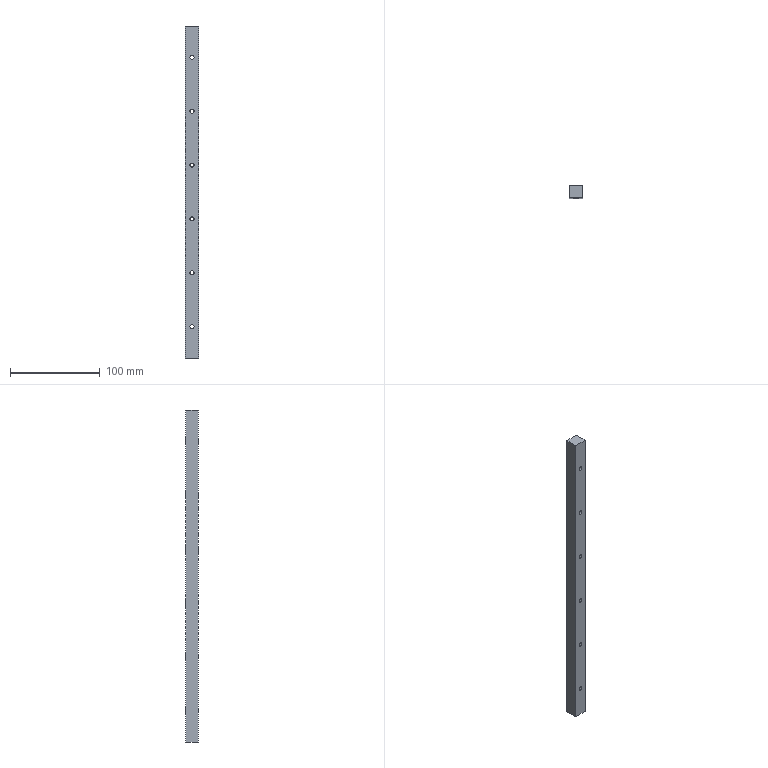Part | STEP file | PN_0038 15 guide rail | 1 solid | 36 faces | box 15 x 14 x 370 mm | volume 75457 mm3 | cylinder 24 | plane 12 | commonest cylinder face diameters 4.5 x12 8 x12